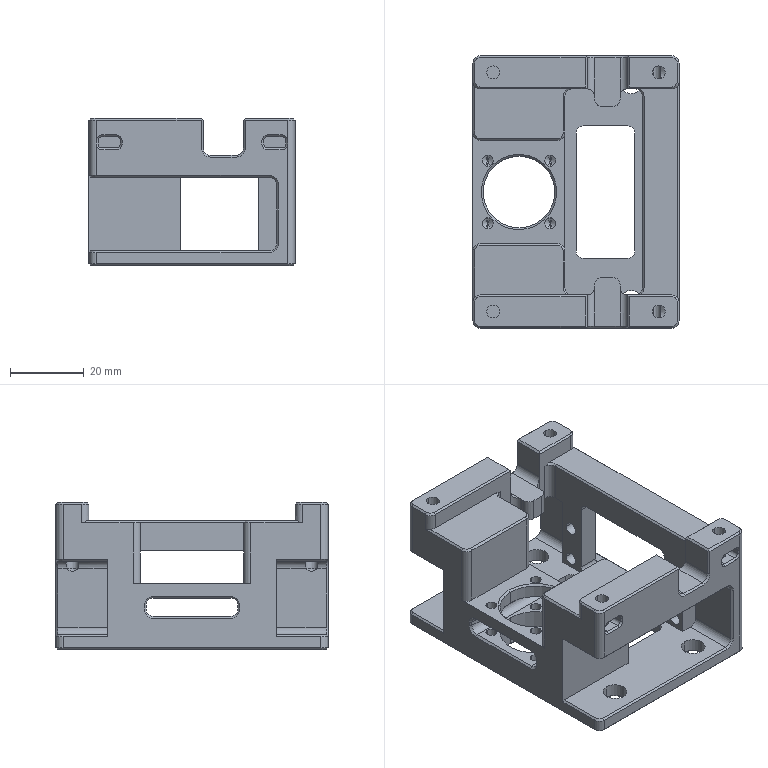CAM job | Mastercam | 3-axis milling, 5-axis milling, drilling | part box 56 x 74 x 40 mm | stock box 64 x 82 x 40 mm
Tools:
tool_number,name,type,diameter_mm,corner_radius_mm,flutes,flute_length_mm,overall_length_mm,shoulder_length_mm,holder_diameter_mm,length_offset,diameter_offset,default_rpm,default_feed_mm_min,default_plunge_mm_min,coolant
2,2 Flat End Mill,end mill,2,0,4,25,75,25,50,2,2,5000,600,600,COOL_OFF
3,3 Flat End Mill,end mill,3,0,4,25,75,25,50,3,3,3333,399.96,600,COOL_OFF
4,4 Flat End Mill,end mill,4,0,4,25,75,25,50,4,4,2500,300,600,COOL_OFF
5,4 Chamfer Mill,chamfer mill,4,0,4,25,75,30,50,5,5,6250,750,600,COOL_OFF
6,6 Flat End Mill,end mill,6,0,4,25,75,25,50,6,6,10000,3000,600,COOL_OFF
8,8 Flat End Mill,end mill,8,0,4,25,75,25,50,8,8,1250,150,600,COOL_OFF
11,12 Flat End Mill,end mill,12,0,4,25,75,25,50,11,11,10000,5000,600,COOL_OFF
12,12 Flat End Mill,end mill,12,0,4,25,75,25,50,12,12,833,99.96,600,COOL_OFF
18,4 Ball Mill / Bull Nose Mill,ball end mill,4,2,4,25,100,30,50,18,18,3000,360,600,COOL_OFF
24,100 Flat End Mill,end mill,100,0,4,25,75,25,50,24,24,100,12,600,COOL_OFF
Operations:
seq,operation,operation_type,tool_number,tool_name,tool_diameter_mm,spindle_rpm,feed_mm_min,plunge_mm_min,retract_mm_min,cycle_time_s,wcs,posted,nc_file
1,Facing - [WCS: Plane] - [Tplane: Plane],Facing,24,100 Flat End Mill,100,4000,1000,600,1200,15.19,Plane,yes,.nc
2,Contour (Ramp) - [WCS: Plane] - [Tplane: Plane],Contour,11,12 Flat End Mill,12,10000,5000,600,1200,147.979,Plane,yes,.nc
3,Contour (2D) - [WCS: Plane] - [Tplane: Plane],Contour,12,12 Flat End Mill,12,7000,1000,600,1200,41.22,Plane,yes,.nc
4,Contour (Ramp) - [WCS: Plane] - [Tplane: Plane],Contour,11,12 Flat End Mill,12,7000,2000,600,1200,28.895,Plane,yes,.nc
5,Contour (2D) - [WCS: Plane] - [Tplane: Plane],Contour,12,12 Flat End Mill,12,7000,1000,600,1200,6.291,Plane,yes,.nc
6,Contour (Ramp) - [WCS: Plane] - [Tplane: Plane],Contour,8,8 Flat End Mill,8,7000,2000,600,1200,29.548,Plane,yes,.nc
7,Contour (Remachining) - [WCS: Plane] - [Tplane: Plane],Contour,4,4 Flat End Mill,4,7000,3000,600,1200,13.445,Plane,yes,.nc
8,Contour (2D) - [WCS: Plane] - [Tplane: Plane],Contour,4,4 Flat End Mill,4,7000,1000,600,1200,6.475,Plane,yes,.nc
9,Contour (Ramp) - [WCS: Plane] - [Tplane: Plane],Contour,4,4 Flat End Mill,4,7000,2000,600,1200,18.175,Plane,yes,.nc
10,Contour (2D) - [WCS: Plane] - [Tplane: Plane],Contour,4,4 Flat End Mill,4,7000,1000,600,1200,9.439,Plane,yes,.nc
11,Contour (2D chamfer) - [WCS: Plane] - [Tplane: Plane],Contour,5,4 Chamfer Mill,4,6000,1000,600,1200,34.613,Plane,yes,.nc
12,Facing - [WCS: Plane-1] - [Tplane: Plane-1],Facing,12,12 Flat End Mill,12,7000,3000,600,1200,200.618,Plane-1,yes,.nc
13,Facing - [WCS: Plane-1] - [Tplane: Plane-1],Facing,24,100 Flat End Mill,100,4000,1000,600,1200,15.79,Plane-1,yes,.nc
14,Contour (2D chamfer) - [WCS: Plane-1] - [Tplane: Plane-1],Contour,5,4 Chamfer Mill,4,6000,1000,600,1200,16.472,Plane-1,yes,.nc
15,3D High Speed (Area roughing) - [WCS: Plane-2] - [Tplane: Plane-2],HighSpeed3D,8,8 Flat End Mill,8,7000,3000,600,1200,94.686,Plane-2,yes,.nc
16,3D High Speed (Waterline rest passes) - [WCS: Plane-2] - [Tplane: Plane-2],HighSpeed3D,4,4 Flat End Mill,4,7000,3000,600,1200,18.731,Plane-2,yes,.nc
17,2D High Speed (2D Area Mill) - [WCS: Plane-2] - [Tplane: Plane-2],HighSpeed2D,4,4 Flat End Mill,4,7000,1000,600,1200,17.768,Plane-2,yes,.nc
18,Contour (2D) - [WCS: Plane-2] - [Tplane: Plane-2],Contour,4,4 Flat End Mill,4,6000,1000,600,1200,9.231,Plane-2,yes,.nc
19,Contour (2D) - [WCS: Plane-2] - [Tplane: Plane-2],Contour,4,4 Flat End Mill,4,7000,1000,600,1200,6.413,Plane-2,yes,.nc
20,Contour (2D chamfer) - [WCS: Plane-2] - [Tplane: Plane-2],Contour,5,4 Chamfer Mill,4,6000,1000,600,1200,9.862,Plane-2,yes,.nc
21,Contour (2D chamfer) - [WCS: Plane-2] - [Tplane: Plane-2],Contour,5,4 Chamfer Mill,4,6000,1000,600,1200,3.53,Plane-2,yes,.nc
22,Drill/Counterbore - [WCS: Plane-2] - [Tplane: Plane-2],Drill,5,4 Chamfer Mill,4,3000,300,600,1200,3.274,Plane-2,yes,.nc
23,Contour (Ramp) - [WCS: Plane-3] - [Tplane: Plane-3],Contour,3,3 Flat End Mill,3,6000,1500,600,1200,198.717,Plane-3,yes,.nc
24,Contour (Ramp) - [WCS: Plane-3] - [Tplane: Plane-3],Contour,3,3 Flat End Mill,3,6000,500,600,1200,56.376,Plane-3,yes,.nc
25,Contour (2D chamfer) - [WCS: Plane-3] - [Tplane: Plane-3],Contour,5,4 Chamfer Mill,4,6000,1000,600,1200,3.982,Plane-3,yes,.nc
26,2D High Speed (2D Area Mill) - [WCS: Plane-4] - [Tplane: Plane-4],HighSpeed2D,8,8 Flat End Mill,8,7000,3000,600,1200,141.704,Plane-4,yes,.nc
27,Contour (Ramp) - [WCS: Plane-4] - [Tplane: Plane-4],Contour,8,8 Flat End Mill,8,7000,2000,600,1200,25.686,Plane-4,yes,.nc
28,Contour (Remachining) - [WCS: Plane-4] - [Tplane: Plane-4],Contour,4,4 Flat End Mill,4,7000,2000,600,1200,18.16,Plane-4,yes,.nc
29,Contour (2D) - [WCS: Plane-4] - [Tplane: Plane-4],Contour,4,4 Flat End Mill,4,7000,1000,600,1200,11.232,Plane-4,yes,.nc
30,Contour (Remachining) - [WCS: Plane-4] - [Tplane: Plane-4],Contour,4,4 Flat End Mill,4,6000,2000,600,1200,21.229,Plane-4,yes,.nc
31,2D High Speed (2D Area Mill) - [WCS: Plane-4] - [Tplane: Plane-4],HighSpeed2D,4,4 Flat End Mill,4,7000,1000,600,1200,31.597,Plane-4,yes,.nc
32,Contour (2D) - [WCS: Plane-4] - [Tplane: Plane-4],Contour,4,4 Flat End Mill,4,7000,800,600,1200,40.56,Plane-4,yes,.nc
33,Contour (Ramp) - [WCS: Plane-4] - [Tplane: Plane-4],Contour,2,2 Flat End Mill,2,7000,1500,600,1200,31.868,Plane-4,yes,.nc
34,Contour (Ramp) - [WCS: Plane-4] - [Tplane: Plane-4],Contour,2,2 Flat End Mill,2,7000,500,600,1200,13.601,Plane-4,yes,.nc
35,Contour (2D chamfer) - [WCS: Plane-4] - [Tplane: Plane-4],Contour,5,4 Chamfer Mill,4,6000,1000,600,1200,13.369,Plane-4,yes,.nc
36,Unified Morph - [WCS: Plane-4] - [Tplane: Plane-4],461,18,4 Ball Mill / Bull Nose Mill,4,7000,3000,600,1200,2.098,Plane-4,yes,.nc
37,Unified Morph - [WCS: Plane-4] - [Tplane: Plane-4],461,18,4 Ball Mill / Bull Nose Mill,4,7000,3000,600,1200,2.068,Plane-4,yes,.nc
38,2D High Speed (2D Area Mill) - [WCS: Plane-5] - [Tplane: Plane-5],HighSpeed2D,8,8 Flat End Mill,8,7000,3000,600,1200,141.704,Plane-5,yes,.nc
39,Contour (Ramp) - [WCS: Plane-5] - [Tplane: Plane-5],Contour,8,8 Flat End Mill,8,7000,2000,600,1200,25.686,Plane-5,yes,.nc
40,Contour (Remachining) - [WCS: Plane-5] - [Tplane: Plane-5],Contour,4,4 Flat End Mill,4,7000,2000,600,1200,18.16,Plane-5,yes,.nc
41,Contour (2D) - [WCS: Plane-5] - [Tplane: Plane-5],Contour,4,4 Flat End Mill,4,7000,1000,600,1200,11.232,Plane-5,yes,.nc
42,Contour (Remachining) - [WCS: Plane-5] - [Tplane: Plane-5],Contour,4,4 Flat End Mill,4,6000,2000,600,1200,21.233,Plane-5,yes,.nc
43,2D High Speed (2D Area Mill) - [WCS: Plane-5] - [Tplane: Plane-5],HighSpeed2D,4,4 Flat End Mill,4,7000,1000,600,1200,31.597,Plane-5,yes,.nc
44,Contour (2D) - [WCS: Plane-5] - [Tplane: Plane-5],Contour,4,4 Flat End Mill,4,7000,800,600,1200,40.56,Plane-5,yes,.nc
45,Contour (Ramp) - [WCS: Plane-5] - [Tplane: Plane-5],Contour,2,2 Flat End Mill,2,7000,1500,600,1200,31.868,Plane-5,yes,.nc
46,Contour (Ramp) - [WCS: Plane-5] - [Tplane: Plane-5],Contour,2,2 Flat End Mill,2,7000,500,600,1200,13.601,Plane-5,yes,.nc
47,Contour (2D chamfer) - [WCS: Plane-5] - [Tplane: Plane-5],Contour,5,4 Chamfer Mill,4,6000,1000,600,1200,13.515,Plane-5,yes,.nc
48,Unified Morph - [WCS: Plane-5] - [Tplane: Plane-5],461,18,4 Ball Mill / Bull Nose Mill,4,7000,3000,600,1200,2.068,Plane-5,yes,.nc
49,Unified Morph - [WCS: Plane-5] - [Tplane: Plane-5],461,18,4 Ball Mill / Bull Nose Mill,4,7000,3000,600,1200,2.098,Plane-5,yes,.nc
50,2D High Speed (2D Area Mill) - [WCS: Plane-1] - [Tplane: Plane-1],HighSpeed2D,8,8 Flat End Mill,8,7000,3000,600,1200,264.493,Plane-1,yes,.nc
51,Contour (2D) - [WCS: Plane-1] - [Tplane: Plane-1],Contour,8,8 Flat End Mill,8,7000,1000,600,1200,11.19,Plane-1,yes,.nc
52,2D High Speed (2D Area Mill) - [WCS: Plane-1] - [Tplane: Plane-1],HighSpeed2D,8,8 Flat End Mill,8,7000,3000,600,1200,295.353,Plane-1,yes,.nc
53,2D High Speed (2D Area Mill) - [WCS: Plane-1] - [Tplane: Plane-1],HighSpeed2D,8,8 Flat End Mill,8,7000,3000,600,1200,245.733,Plane-1,yes,.nc
54,Contour (2D) - [WCS: Plane-1] - [Tplane: Plane-1],Contour,8,8 Flat End Mill,8,7000,1000,600,1200,10.085,Plane-1,yes,.nc
55,Contour (Remachining) - [WCS: Plane-1] - [Tplane: Plane-1],Contour,4,4 Flat End Mill,4,5000,2000,600,1200,205.307,Plane-1,yes,.nc
56,Contour (Ramp) - [WCS: Plane-1] - [Tplane: Plane-1],Contour,4,4 Flat End Mill,4,5000,800,600,1200,99.363,Plane-1,yes,.nc
57,2D High Speed (2D Area Mill) - [WCS: Plane-1] - [Tplane: Plane-1],HighSpeed2D,4,4 Flat End Mill,4,5000,800,600,1200,46.904,Plane-1,yes,.nc
58,Contour (2D chamfer) - [WCS: Plane-1] - [Tplane: Plane-1],Contour,5,4 Chamfer Mill,4,6000,1000,600,1200,8.846,Plane-1,yes,.nc
59,Contour (2D chamfer) - [WCS: Plane-1] - [Tplane: Plane-1],Contour,5,4 Chamfer Mill,4,6000,1000,600,1200,14.908,Plane-1,yes,.nc
60,Contour (2D chamfer) - [WCS: Plane-1] - [Tplane: Plane-1],Contour,5,4 Chamfer Mill,4,6000,1000,600,1200,4.475,Plane-1,yes,.nc
61,Drill/Counterbore - [WCS: Plane-1] - [Tplane: Plane-1],Drill,5,4 Chamfer Mill,4,3000,300,600,1200,6.884,Plane-1,yes,.nc
62,Facing - [WCS: Plane] - [Tplane: Plane],Facing,24,100 Flat End Mill,100,4000,1000,600,1200,15.19,Plane,yes,.nc
63,Contour (Ramp) - [WCS: Plane] - [Tplane: Plane],Contour,11,12 Flat End Mill,12,10000,5000,600,1200,147.979,Plane,yes,.nc
64,Contour (2D) - [WCS: Plane] - [Tplane: Plane],Contour,12,12 Flat End Mill,12,7000,1000,600,1200,119.521,Plane,yes,.nc
65,Contour (Ramp) - [WCS: Plane] - [Tplane: Plane],Contour,11,12 Flat End Mill,12,7000,2000,600,1200,28.895,Plane,yes,.nc
66,Contour (2D) - [WCS: Plane] - [Tplane: Plane],Contour,12,12 Flat End Mill,12,7000,1000,600,1200,6.291,Plane,yes,.nc
67,Contour (Ramp) - [WCS: Plane] - [Tplane: Plane],Contour,8,8 Flat End Mill,8,7000,2000,600,1200,29.548,Plane,yes,.nc
68,Contour (Remachining) - [WCS: Plane] - [Tplane: Plane],Contour,4,4 Flat End Mill,4,7000,3000,600,1200,13.445,Plane,yes,.nc
69,Contour (2D) - [WCS: Plane] - [Tplane: Plane],Contour,4,4 Flat End Mill,4,7000,1000,600,1200,6.475,Plane,yes,.nc
70,Helix Bore - [WCS: Plane] - [Tplane: Plane],HelixBore,6,6 Flat End Mill,6,10000,3000,600,1200,42.412,Plane,yes,.nc
71,Contour (2D chamfer) - [WCS: Plane] - [Tplane: Plane],Contour,5,4 Chamfer Mill,4,6000,1000,600,1200,27.359,Plane,yes,.nc
72,Contour (2D chamfer) - [WCS: Plane] - [Tplane: Plane],Contour,5,4 Chamfer Mill,4,6000,1000,600,1200,9.893,Plane,yes,.nc
73,Facing - [WCS: Plane-1] - [Tplane: Plane-1],Facing,12,12 Flat End Mill,12,7000,3000,600,1200,200.618,Plane-1,yes,.nc
74,Facing - [WCS: Plane-1] - [Tplane: Plane-1],Facing,24,100 Flat End Mill,100,4000,1000,600,1200,15.79,Plane-1,yes,.nc
75,Contour (2D chamfer) - [WCS: Plane-1] - [Tplane: Plane-1],Contour,5,4 Chamfer Mill,4,6000,1000,600,1200,16.472,Plane-1,yes,.nc
76,3D High Speed (Area roughing) - [WCS: Plane-2] - [Tplane: Plane-2],HighSpeed3D,8,8 Flat End Mill,8,7000,3000,600,1200,90.554,Plane-2,yes,.nc
77,3D High Speed (Waterline rest passes) - [WCS: Plane-2] - [Tplane: Plane-2],HighSpeed3D,4,4 Flat End Mill,4,7000,3000,600,1200,19.062,Plane-2,yes,.nc
78,2D High Speed (2D Area Mill) - [WCS: Plane-2] - [Tplane: Plane-2],HighSpeed2D,4,4 Flat End Mill,4,7000,1000,600,1200,17.749,Plane-2,yes,.nc
79,Contour (2D) - [WCS: Plane-2] - [Tplane: Plane-2],Contour,4,4 Flat End Mill,4,6000,1000,600,1200,9.221,Plane-2,yes,.nc
80,Contour (2D) - [WCS: Plane-2] - [Tplane: Plane-2],Contour,4,4 Flat End Mill,4,7000,1000,600,1200,6.413,Plane-2,yes,.nc
81,Contour (2D chamfer) - [WCS: Plane-2] - [Tplane: Plane-2],Contour,5,4 Chamfer Mill,4,6000,1000,600,1200,9.862,Plane-2,yes,.nc
82,Contour (2D chamfer) - [WCS: Plane-2] - [Tplane: Plane-2],Contour,5,4 Chamfer Mill,4,6000,1000,600,1200,3.415,Plane-2,yes,.nc
83,Drill/Counterbore - [WCS: Plane-2] - [Tplane: Plane-2],Drill,5,4 Chamfer Mill,4,3000,300,600,1200,3.274,Plane-2,yes,.nc
84,2D High Speed (2D Area Mill) - [WCS: Plane-4] - [Tplane: Plane-4],HighSpeed2D,8,8 Flat End Mill,8,7000,3000,600,1200,146.709,Plane-4,yes,.nc
85,Contour (Ramp) - [WCS: Plane-4] - [Tplane: Plane-4],Contour,8,8 Flat End Mill,8,7000,2000,600,1200,25.686,Plane-4,yes,.nc
86,Contour (Remachining) - [WCS: Plane-4] - [Tplane: Plane-4],Contour,4,4 Flat End Mill,4,7000,2000,600,1200,18.16,Plane-4,yes,.nc
87,Contour (2D) - [WCS: Plane-4] - [Tplane: Plane-4],Contour,4,4 Flat End Mill,4,7000,1000,600,1200,11.232,Plane-4,yes,.nc
88,Contour (Remachining) - [WCS: Plane-4] - [Tplane: Plane-4],Contour,4,4 Flat End Mill,4,6000,2000,600,1200,21.217,Plane-4,yes,.nc
89,2D High Speed (2D Area Mill) - [WCS: Plane-4] - [Tplane: Plane-4],HighSpeed2D,4,4 Flat End Mill,4,7000,1000,600,1200,32.701,Plane-4,yes,.nc
90,Contour (2D) - [WCS: Plane-4] - [Tplane: Plane-4],Contour,4,4 Flat End Mill,4,7000,800,600,1200,41.789,Plane-4,yes,.nc
91,Contour (2D chamfer) - [WCS: Plane-4] - [Tplane: Plane-4],Contour,5,4 Chamfer Mill,4,6000,1000,600,1200,10.602,Plane-4,yes,.nc
92,Unified Morph - [WCS: Plane-4] - [Tplane: Plane-4],461,18,4 Ball Mill / Bull Nose Mill,4,7000,3000,600,1200,2.098,Plane-4,yes,.nc
93,Unified Morph - [WCS: Plane-4] - [Tplane: Plane-4],461,18,4 Ball Mill / Bull Nose Mill,4,7000,3000,600,1200,1.987,Plane-4,yes,.nc
94,2D High Speed (2D Area Mill) - [WCS: Plane-5] - [Tplane: Plane-5],HighSpeed2D,8,8 Flat End Mill,8,7000,3000,600,1200,146.709,Plane-5,yes,.nc
95,Contour (Ramp) - [WCS: Plane-5] - [Tplane: Plane-5],Contour,8,8 Flat End Mill,8,7000,2000,600,1200,25.686,Plane-5,yes,.nc
96,Contour (Remachining) - [WCS: Plane-5] - [Tplane: Plane-5],Contour,4,4 Flat End Mill,4,7000,2000,600,1200,18.16,Plane-5,yes,.nc
97,Contour (2D) - [WCS: Plane-5] - [Tplane: Plane-5],Contour,4,4 Flat End Mill,4,7000,1000,600,1200,11.232,Plane-5,yes,.nc
98,Contour (Remachining) - [WCS: Plane-5] - [Tplane: Plane-5],Contour,4,4 Flat End Mill,4,6000,2000,600,1200,21.243,Plane-5,yes,.nc
99,2D High Speed (2D Area Mill) - [WCS: Plane-5] - [Tplane: Plane-5],HighSpeed2D,4,4 Flat End Mill,4,7000,1000,600,1200,32.701,Plane-5,yes,.nc
100,Contour (2D) - [WCS: Plane-5] - [Tplane: Plane-5],Contour,4,4 Flat End Mill,4,7000,800,600,1200,41.789,Plane-5,yes,.nc
101,Contour (2D chamfer) - [WCS: Plane-5] - [Tplane: Plane-5],Contour,5,4 Chamfer Mill,4,6000,1000,600,1200,10.749,Plane-5,yes,.nc
102,Unified Morph - [WCS: Plane-5] - [Tplane: Plane-5],461,18,4 Ball Mill / Bull Nose Mill,4,7000,3000,600,1200,2.068,Plane-5,yes,.nc
103,Unified Morph - [WCS: Plane-5] - [Tplane: Plane-5],461,18,4 Ball Mill / Bull Nose Mill,4,7000,3000,600,1200,2.098,Plane-5,yes,.nc
104,2D High Speed (2D Area Mill) - [WCS: Plane-1] - [Tplane: Plane-1],HighSpeed2D,8,8 Flat End Mill,8,7000,3000,600,1200,264.493,Plane-1,yes,.nc
105,Contour (2D) - [WCS: Plane-1] - [Tplane: Plane-1],Contour,8,8 Flat End Mill,8,7000,1000,600,1200,11.19,Plane-1,yes,.nc
106,2D High Speed (2D Area Mill) - [WCS: Plane-1] - [Tplane: Plane-1],HighSpeed2D,8,8 Flat End Mill,8,7000,3000,600,1200,295.353,Plane-1,yes,.nc
107,2D High Speed (2D Area Mill) - [WCS: Plane-1] - [Tplane: Plane-1],HighSpeed2D,8,8 Flat End Mill,8,7000,3000,600,1200,245.733,Plane-1,yes,.nc
108,Contour (2D) - [WCS: Plane-1] - [Tplane: Plane-1],Contour,8,8 Flat End Mill,8,7000,1000,600,1200,10.085,Plane-1,yes,.nc
109,Contour (Remachining) - [WCS: Plane-1] - [Tplane: Plane-1],Contour,4,4 Flat End Mill,4,5000,2000,600,1200,205.307,Plane-1,yes,.nc
110,Contour (Ramp) - [WCS: Plane-1] - [Tplane: Plane-1],Contour,4,4 Flat End Mill,4,5000,800,600,1200,99.363,Plane-1,yes,.nc
111,2D High Speed (2D Area Mill) - [WCS: Plane-1] - [Tplane: Plane-1],HighSpeed2D,4,4 Flat End Mill,4,5000,800,600,1200,46.904,Plane-1,yes,.nc
112,Contour (2D chamfer) - [WCS: Plane-1] - [Tplane: Plane-1],Contour,5,4 Chamfer Mill,4,6000,1000,600,1200,8.846,Plane-1,yes,.nc
113,Contour (2D chamfer) - [WCS: Plane-1] - [Tplane: Plane-1],Contour,5,4 Chamfer Mill,4,6000,1000,600,1200,14.908,Plane-1,yes,.nc
114,Contour (2D chamfer) - [WCS: Plane-1] - [Tplane: Plane-1],Contour,5,4 Chamfer Mill,4,6000,1000,600,1200,4.475,Plane-1,yes,.nc
115,Drill/Counterbore - [WCS: Plane-1] - [Tplane: Plane-1],Drill,5,4 Chamfer Mill,4,3000,300,600,1200,6.884,Plane-1,yes,.nc